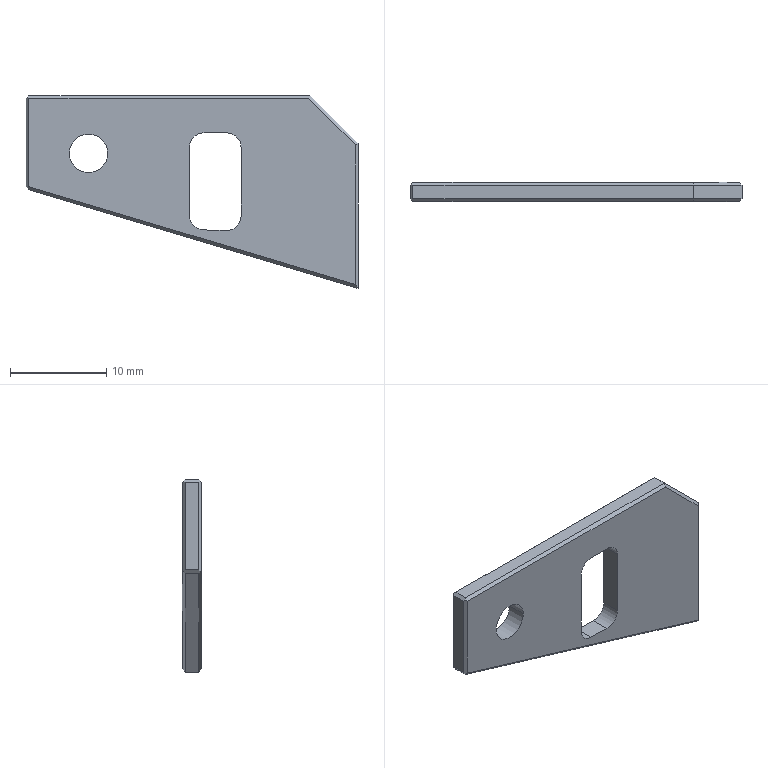Part | NX | 1 solid | 29 faces | box 34.5 x 2 x 20.034 mm | volume 861.777 mm3 | plane 23 | cylinder 6 | commonest cylinder face diameters 3 x4 4 x2
STEP:
#1=CARTESIAN_POINT('',(-158.,158.2,-56.284));
#2=VERTEX_POINT('',#1);
#3=CARTESIAN_POINT('',(-158.,156.8,-56.284));
#4=VERTEX_POINT('',#3);
#5=CARTESIAN_POINT('',(-158.,157.5,-56.284));
#6=DIRECTION('',(0.,-1.,0.));
#7=VECTOR('',#6,1000.);
#8=LINE('',#5,#7);
#9=EDGE_CURVE('',#2,#4,#8,.T.);
#10=ORIENTED_EDGE('',*,*,#9,.T.);
#11=CARTESIAN_POINT('',(-158.,156.8,-47.2));
#12=VERTEX_POINT('',#11);
#13=CARTESIAN_POINT('',(-158.,156.8,-58.685));
#14=DIRECTION('',(0.,0.,1.));
#15=VECTOR('',#14,1000.);
#16=LINE('',#13,#15);
#17=EDGE_CURVE('',#4,#12,#16,.T.);
#18=ORIENTED_EDGE('',*,*,#17,.T.);
#19=CARTESIAN_POINT('',(-158.,158.2,-47.2));
#20=VERTEX_POINT('',#19);
#21=CARTESIAN_POINT('',(-158.,157.5,-47.2));
#22=DIRECTION('',(0.,1.,0.));
#23=VECTOR('',#22,1000.);
#24=LINE('',#21,#23);
#25=EDGE_CURVE('',#12,#20,#24,.T.);
#26=ORIENTED_EDGE('',*,*,#25,.T.);
#27=CARTESIAN_POINT('',(-158.,158.2,-58.685));
#28=DIRECTION('',(0.,0.,1.));
#29=VECTOR('',#28,1000.);
#30=LINE('',#27,#29);
#31=EDGE_CURVE('',#2,#20,#30,.T.);
#32=ORIENTED_EDGE('',*,*,#31,.F.);
#33=EDGE_LOOP('',(#10,#18,#26,#32));
#34=FACE_BOUND('',#33,.T.);
#35=CARTESIAN_POINT('',(-158.,156.5,-42.9));
#36=DIRECTION('',(-1.,0.,0.));
#37=DIRECTION('',(0.,0.,1.));
#38=AXIS2_PLACEMENT_3D('',#35,#36,#37);
#39=PLANE('',#38);
#40=ADVANCED_FACE('',(#34),#39,.T.);
#41=CARTESIAN_POINT('',(-128.5,156.8,-46.9));
#42=VERTEX_POINT('',#41);
#43=CARTESIAN_POINT('',(-128.5,158.2,-46.9));
#44=VERTEX_POINT('',#43);
#45=CARTESIAN_POINT('',(-128.5,157.5,-46.9));
#46=DIRECTION('',(0.,1.,0.));
#47=VECTOR('',#46,1000.);
#48=LINE('',#45,#47);
#49=EDGE_CURVE('',#42,#44,#48,.T.);
#50=ORIENTED_EDGE('',*,*,#49,.T.);
#51=CARTESIAN_POINT('',(-157.7,158.2,-46.9));
#52=VERTEX_POINT('',#51);
#53=CARTESIAN_POINT('',(-143.25,158.2,-46.9));
#54=DIRECTION('',(1.,0.,0.));
#55=VECTOR('',#54,1000.);
#56=LINE('',#53,#55);
#57=EDGE_CURVE('',#52,#44,#56,.T.);
#58=ORIENTED_EDGE('',*,*,#57,.F.);
#59=CARTESIAN_POINT('',(-157.7,156.8,-46.9));
#60=VERTEX_POINT('',#59);
#61=CARTESIAN_POINT('',(-157.7,157.5,-46.9));
#62=DIRECTION('',(0.,1.,0.));
#63=VECTOR('',#62,1000.);
#64=LINE('',#61,#63);
#65=EDGE_CURVE('',#60,#52,#64,.T.);
#66=ORIENTED_EDGE('',*,*,#65,.F.);
#67=CARTESIAN_POINT('',(-143.25,156.8,-46.9));
#68=DIRECTION('',(1.,0.,0.));
#69=VECTOR('',#68,1000.);
#70=LINE('',#67,#69);
#71=EDGE_CURVE('',#60,#42,#70,.T.);
#72=ORIENTED_EDGE('',*,*,#71,.T.);
#73=EDGE_LOOP('',(#50,#58,#66,#72));
#74=FACE_BOUND('',#73,.T.);
#75=CARTESIAN_POINT('',(-123.5,156.5,-46.9));
#76=DIRECTION('',(0.,0.,1.));
#77=DIRECTION('',(0.,-1.,0.));
#78=AXIS2_PLACEMENT_3D('',#75,#76,#77);
#79=PLANE('',#78);
#80=ADVANCED_FACE('',(#74),#79,.T.);
#81=CARTESIAN_POINT('',(-123.5,158.2,-51.9));
#82=VERTEX_POINT('',#81);
#83=CARTESIAN_POINT('',(-123.5,158.2,-66.934));
#84=VERTEX_POINT('',#83);
#85=CARTESIAN_POINT('',(-123.5,158.2,-58.685));
#86=DIRECTION('',(0.,0.,-1.));
#87=VECTOR('',#86,1000.);
#88=LINE('',#85,#87);
#89=EDGE_CURVE('',#82,#84,#88,.T.);
#90=ORIENTED_EDGE('',*,*,#89,.F.);
#91=CARTESIAN_POINT('',(-123.5,156.8,-51.9));
#92=VERTEX_POINT('',#91);
#93=CARTESIAN_POINT('',(-123.5,157.5,-51.9));
#94=DIRECTION('',(0.,1.,0.));
#95=VECTOR('',#94,1000.);
#96=LINE('',#93,#95);
#97=EDGE_CURVE('',#92,#82,#96,.T.);
#98=ORIENTED_EDGE('',*,*,#97,.F.);
#99=CARTESIAN_POINT('',(-123.5,156.8,-66.934));
#100=VERTEX_POINT('',#99);
#101=CARTESIAN_POINT('',(-123.5,156.8,-58.685));
#102=DIRECTION('',(0.,0.,-1.));
#103=VECTOR('',#102,1000.);
#104=LINE('',#101,#103);
#105=EDGE_CURVE('',#92,#100,#104,.T.);
#106=ORIENTED_EDGE('',*,*,#105,.T.);
#107=CARTESIAN_POINT('',(-123.5,156.5,-66.934));
#108=DIRECTION('',(0.,1.,0.));
#109=VECTOR('',#108,1000.);
#110=LINE('',#107,#109);
#111=EDGE_CURVE('',#100,#84,#110,.T.);
#112=ORIENTED_EDGE('',*,*,#111,.T.);
#113=EDGE_LOOP('',(#90,#98,#106,#112));
#114=FACE_BOUND('',#113,.T.);
#115=CARTESIAN_POINT('',(-123.5,156.5,-67.9));
#116=DIRECTION('',(1.,0.,0.));
#117=DIRECTION('',(0.,1.,0.));
#118=AXIS2_PLACEMENT_3D('',#115,#116,#117);
#119=PLANE('',#118);
#120=ADVANCED_FACE('',(#114),#119,.T.);
#121=CARTESIAN_POINT('',(-135.65,156.5,-59.427));
#122=VERTEX_POINT('',#121);
#123=CARTESIAN_POINT('',(-135.65,158.5,-59.427));
#124=VERTEX_POINT('',#123);
#125=CARTESIAN_POINT('',(-135.65,156.5,-59.427));
#126=DIRECTION('',(0.,1.,0.));
#127=VECTOR('',#126,1000.);
#128=LINE('',#125,#127);
#129=EDGE_CURVE('',#122,#124,#128,.T.);
#130=ORIENTED_EDGE('',*,*,#129,.T.);
#131=CARTESIAN_POINT('',(-137.197,158.5,-60.926));
#132=VERTEX_POINT('',#131);
#133=CARTESIAN_POINT('',(-137.15,158.5,-59.427));
#134=DIRECTION('',(0.,1.,0.));
#135=DIRECTION('',(-1.,0.,0.));
#136=AXIS2_PLACEMENT_3D('',#133,#134,#135);
#137=CIRCLE('',#136,1.5);
#138=EDGE_CURVE('',#124,#132,#137,.T.);
#139=ORIENTED_EDGE('',*,*,#138,.T.);
#140=CARTESIAN_POINT('',(-137.197,156.5,-60.926));
#141=VERTEX_POINT('',#140);
#142=CARTESIAN_POINT('',(-137.197,156.5,-60.926));
#143=DIRECTION('',(0.,1.,0.));
#144=VECTOR('',#143,1000.);
#145=LINE('',#142,#144);
#146=EDGE_CURVE('',#141,#132,#145,.T.);
#147=ORIENTED_EDGE('',*,*,#146,.F.);
#148=CARTESIAN_POINT('',(-137.15,156.5,-59.427));
#149=DIRECTION('',(0.,1.,0.));
#150=DIRECTION('',(-1.,0.,0.));
#151=AXIS2_PLACEMENT_3D('',#148,#149,#150);
#152=CIRCLE('',#151,1.5);
#153=EDGE_CURVE('',#122,#141,#152,.T.);
#154=ORIENTED_EDGE('',*,*,#153,.F.);
#155=EDGE_LOOP('',(#130,#139,#147,#154));
#156=FACE_BOUND('',#155,.T.);
#157=CARTESIAN_POINT('',(-137.15,156.5,-59.427));
#158=DIRECTION('',(0.,1.,0.));
#159=DIRECTION('',(-1.,0.,0.));
#160=AXIS2_PLACEMENT_3D('',#157,#158,#159);
#161=CYLINDRICAL_SURFACE('',#160,1.5);
#162=ADVANCED_FACE('',(#156),#161,.F.);
#163=ORIENTED_EDGE('',*,*,#111,.F.);
#164=CARTESIAN_POINT('',(-157.713,156.8,-56.67));
#165=VERTEX_POINT('',#164);
#166=CARTESIAN_POINT('',(-140.75,156.8,-61.759));
#167=DIRECTION('',(-0.9578,0.,0.2873));
#168=VECTOR('',#167,1000.);
#169=LINE('',#166,#168);
#170=EDGE_CURVE('',#100,#165,#169,.T.);
#171=ORIENTED_EDGE('',*,*,#170,.T.);
#172=CARTESIAN_POINT('',(-157.713,158.2,-56.67));
#173=VERTEX_POINT('',#172);
#174=CARTESIAN_POINT('',(-157.713,157.5,-56.67));
#175=DIRECTION('',(0.,-1.,0.));
#176=VECTOR('',#175,1000.);
#177=LINE('',#174,#176);
#178=EDGE_CURVE('',#173,#165,#177,.T.);
#179=ORIENTED_EDGE('',*,*,#178,.F.);
#180=CARTESIAN_POINT('',(-140.75,158.2,-61.759));
#181=DIRECTION('',(-0.9578,0.,0.2873));
#182=VECTOR('',#181,1000.);
#183=LINE('',#180,#182);
#184=EDGE_CURVE('',#84,#173,#183,.T.);
#185=ORIENTED_EDGE('',*,*,#184,.F.);
#186=EDGE_LOOP('',(#163,#171,#179,#185));
#187=FACE_BOUND('',#186,.T.);
#188=CARTESIAN_POINT('',(-160.069,156.5,-55.963));
#189=DIRECTION('',(-0.2873,0.,-0.9578));
#190=DIRECTION('',(-0.9578,0.,0.2873));
#191=AXIS2_PLACEMENT_3D('',#188,#189,#190);
#192=PLANE('',#191);
#193=ADVANCED_FACE('',(#187),#192,.T.);
#194=CARTESIAN_POINT('',(-141.001,156.5,-59.354));
#195=VERTEX_POINT('',#194);
#196=CARTESIAN_POINT('',(-141.001,158.5,-59.354));
#197=VERTEX_POINT('',#196);
#198=CARTESIAN_POINT('',(-141.001,156.5,-59.354));
#199=DIRECTION('',(0.,1.,0.));
#200=VECTOR('',#199,1000.);
#201=LINE('',#198,#200);
#202=EDGE_CURVE('',#195,#197,#201,.T.);
#203=ORIENTED_EDGE('',*,*,#202,.F.);
#204=CARTESIAN_POINT('',(-139.548,156.5,-60.853));
#205=VERTEX_POINT('',#204);
#206=CARTESIAN_POINT('',(-139.501,156.5,-59.354));
#207=DIRECTION('',(0.,1.,0.));
#208=DIRECTION('',(-1.,0.,0.));
#209=AXIS2_PLACEMENT_3D('',#206,#207,#208);
#210=CIRCLE('',#209,1.5);
#211=EDGE_CURVE('',#205,#195,#210,.T.);
#212=ORIENTED_EDGE('',*,*,#211,.F.);
#213=CARTESIAN_POINT('',(-139.548,158.5,-60.853));
#214=VERTEX_POINT('',#213);
#215=CARTESIAN_POINT('',(-139.548,156.5,-60.853));
#216=DIRECTION('',(0.,1.,0.));
#217=VECTOR('',#216,1000.);
#218=LINE('',#215,#217);
#219=EDGE_CURVE('',#205,#214,#218,.T.);
#220=ORIENTED_EDGE('',*,*,#219,.T.);
#221=CARTESIAN_POINT('',(-139.501,158.5,-59.354));
#222=DIRECTION('',(0.,1.,0.));
#223=DIRECTION('',(-1.,0.,0.));
#224=AXIS2_PLACEMENT_3D('',#221,#222,#223);
#225=CIRCLE('',#224,1.5);
#226=EDGE_CURVE('',#214,#197,#225,.T.);
#227=ORIENTED_EDGE('',*,*,#226,.T.);
#228=EDGE_LOOP('',(#203,#212,#220,#227));
#229=FACE_BOUND('',#228,.T.);
#230=CARTESIAN_POINT('',(-139.501,156.5,-59.354));
#231=DIRECTION('',(0.,1.,0.));
#232=DIRECTION('',(-1.,0.,0.));
#233=AXIS2_PLACEMENT_3D('',#230,#231,#232);
#234=CYLINDRICAL_SURFACE('',#233,1.5);
#235=ADVANCED_FACE('',(#229),#234,.F.);
#236=CARTESIAN_POINT('',(-137.15,156.5,-50.763));
#237=VERTEX_POINT('',#236);
#238=CARTESIAN_POINT('',(-137.15,158.5,-50.763));
#239=VERTEX_POINT('',#238);
#240=CARTESIAN_POINT('',(-137.15,156.5,-50.763));
#241=DIRECTION('',(0.,1.,0.));
#242=VECTOR('',#241,1000.);
#243=LINE('',#240,#242);
#244=EDGE_CURVE('',#237,#239,#243,.T.);
#245=ORIENTED_EDGE('',*,*,#244,.F.);
#246=CARTESIAN_POINT('',(-139.501,156.5,-50.763));
#247=VERTEX_POINT('',#246);
#248=CARTESIAN_POINT('',(-108.092,156.5,-50.763));
#249=DIRECTION('',(1.,0.,0.));
#250=VECTOR('',#249,1000.);
#251=LINE('',#248,#250);
#252=EDGE_CURVE('',#247,#237,#251,.T.);
#253=ORIENTED_EDGE('',*,*,#252,.F.);
#254=CARTESIAN_POINT('',(-139.501,158.5,-50.763));
#255=VERTEX_POINT('',#254);
#256=CARTESIAN_POINT('',(-139.501,156.5,-50.763));
#257=DIRECTION('',(0.,1.,0.));
#258=VECTOR('',#257,1000.);
#259=LINE('',#256,#258);
#260=EDGE_CURVE('',#247,#255,#259,.T.);
#261=ORIENTED_EDGE('',*,*,#260,.T.);
#262=CARTESIAN_POINT('',(-108.092,158.5,-50.763));
#263=DIRECTION('',(1.,0.,0.));
#264=VECTOR('',#263,1000.);
#265=LINE('',#262,#264);
#266=EDGE_CURVE('',#255,#239,#265,.T.);
#267=ORIENTED_EDGE('',*,*,#266,.T.);
#268=EDGE_LOOP('',(#245,#253,#261,#267));
#269=FACE_BOUND('',#268,.T.);
#270=CARTESIAN_POINT('',(-135.65,156.3,-50.763));
#271=DIRECTION('',(0.,0.,1.));
#272=DIRECTION('',(0.,-1.,0.));
#273=AXIS2_PLACEMENT_3D('',#270,#271,#272);
#274=PLANE('',#273);
#275=ADVANCED_FACE('',(#269),#274,.F.);
#276=ORIENTED_EDGE('',*,*,#129,.F.);
#277=CARTESIAN_POINT('',(-135.65,156.5,-52.263));
#278=VERTEX_POINT('',#277);
#279=CARTESIAN_POINT('',(-135.65,156.5,-58.685));
#280=DIRECTION('',(0.,0.,-1.));
#281=VECTOR('',#280,1000.);
#282=LINE('',#279,#281);
#283=EDGE_CURVE('',#278,#122,#282,.T.);
#284=ORIENTED_EDGE('',*,*,#283,.F.);
#285=CARTESIAN_POINT('',(-135.65,158.5,-52.263));
#286=VERTEX_POINT('',#285);
#287=CARTESIAN_POINT('',(-135.65,156.5,-52.263));
#288=DIRECTION('',(0.,1.,0.));
#289=VECTOR('',#288,1000.);
#290=LINE('',#287,#289);
#291=EDGE_CURVE('',#278,#286,#290,.T.);
#292=ORIENTED_EDGE('',*,*,#291,.T.);
#293=CARTESIAN_POINT('',(-135.65,158.5,-58.685));
#294=DIRECTION('',(0.,0.,-1.));
#295=VECTOR('',#294,1000.);
#296=LINE('',#293,#295);
#297=EDGE_CURVE('',#286,#124,#296,.T.);
#298=ORIENTED_EDGE('',*,*,#297,.T.);
#299=EDGE_LOOP('',(#276,#284,#292,#298));
#300=FACE_BOUND('',#299,.T.);
#301=CARTESIAN_POINT('',(-135.65,156.3,-60.975));
#302=DIRECTION('',(1.,0.,0.));
#303=DIRECTION('',(0.,0.,-1.));
#304=AXIS2_PLACEMENT_3D('',#301,#302,#303);
#305=PLANE('',#304);
#306=ADVANCED_FACE('',(#300),#305,.F.);
#307=CARTESIAN_POINT('',(-108.092,158.5,-61.836));
#308=DIRECTION('',(-0.9995,0.,0.03124));
#309=VECTOR('',#308,1000.);
#310=LINE('',#307,#309);
#311=EDGE_CURVE('',#132,#214,#310,.T.);
#312=ORIENTED_EDGE('',*,*,#311,.T.);
#313=ORIENTED_EDGE('',*,*,#219,.F.);
#314=CARTESIAN_POINT('',(-108.092,156.5,-61.836));
#315=DIRECTION('',(-0.9995,0.,0.03124));
#316=VECTOR('',#315,1000.);
#317=LINE('',#314,#316);
#318=EDGE_CURVE('',#141,#205,#317,.T.);
#319=ORIENTED_EDGE('',*,*,#318,.F.);
#320=ORIENTED_EDGE('',*,*,#146,.T.);
#321=EDGE_LOOP('',(#312,#313,#319,#320));
#322=FACE_BOUND('',#321,.T.);
#323=CARTESIAN_POINT('',(-141.001,156.3,-60.807));
#324=DIRECTION('',(-0.03124,0.,-0.9995));
#325=DIRECTION('',(-0.9995,0.,0.03124));
#326=AXIS2_PLACEMENT_3D('',#323,#324,#325);
#327=PLANE('',#326);
#328=ADVANCED_FACE('',(#322),#327,.F.);
#329=ORIENTED_EDGE('',*,*,#202,.T.);
#330=CARTESIAN_POINT('',(-141.001,158.5,-52.263));
#331=VERTEX_POINT('',#330);
#332=CARTESIAN_POINT('',(-141.001,158.5,-58.685));
#333=DIRECTION('',(0.,0.,1.));
#334=VECTOR('',#333,1000.);
#335=LINE('',#332,#334);
#336=EDGE_CURVE('',#197,#331,#335,.T.);
#337=ORIENTED_EDGE('',*,*,#336,.T.);
#338=CARTESIAN_POINT('',(-141.001,156.5,-52.263));
#339=VERTEX_POINT('',#338);
#340=CARTESIAN_POINT('',(-141.001,156.5,-52.263));
#341=DIRECTION('',(0.,1.,0.));
#342=VECTOR('',#341,1000.);
#343=LINE('',#340,#342);
#344=EDGE_CURVE('',#339,#331,#343,.T.);
#345=ORIENTED_EDGE('',*,*,#344,.F.);
#346=CARTESIAN_POINT('',(-141.001,156.5,-58.685));
#347=DIRECTION('',(0.,0.,1.));
#348=VECTOR('',#347,1000.);
#349=LINE('',#346,#348);
#350=EDGE_CURVE('',#195,#339,#349,.T.);
#351=ORIENTED_EDGE('',*,*,#350,.F.);
#352=EDGE_LOOP('',(#329,#337,#345,#351));
#353=FACE_BOUND('',#352,.T.);
#354=CARTESIAN_POINT('',(-141.001,156.3,-50.763));
#355=DIRECTION('',(-1.,0.,0.));
#356=DIRECTION('',(0.,0.,1.));
#357=AXIS2_PLACEMENT_3D('',#354,#355,#356);
#358=PLANE('',#357);
#359=ADVANCED_FACE('',(#353),#358,.F.);
#360=ORIENTED_EDGE('',*,*,#344,.T.);
#361=CARTESIAN_POINT('',(-139.501,158.5,-52.263));
#362=DIRECTION('',(0.,1.,0.));
#363=DIRECTION('',(-1.,0.,0.));
#364=AXIS2_PLACEMENT_3D('',#361,#362,#363);
#365=CIRCLE('',#364,1.5);
#366=EDGE_CURVE('',#331,#255,#365,.T.);
#367=ORIENTED_EDGE('',*,*,#366,.T.);
#368=ORIENTED_EDGE('',*,*,#260,.F.);
#369=CARTESIAN_POINT('',(-139.501,156.5,-52.263));
#370=DIRECTION('',(0.,1.,0.));
#371=DIRECTION('',(-1.,0.,0.));
#372=AXIS2_PLACEMENT_3D('',#369,#370,#371);
#373=CIRCLE('',#372,1.5);
#374=EDGE_CURVE('',#339,#247,#373,.T.);
#375=ORIENTED_EDGE('',*,*,#374,.F.);
#376=EDGE_LOOP('',(#360,#367,#368,#375));
#377=FACE_BOUND('',#376,.T.);
#378=CARTESIAN_POINT('',(-139.501,156.5,-52.263));
#379=DIRECTION('',(0.,1.,0.));
#380=DIRECTION('',(-1.,0.,0.));
#381=AXIS2_PLACEMENT_3D('',#378,#379,#380);
#382=CYLINDRICAL_SURFACE('',#381,1.5);
#383=ADVANCED_FACE('',(#377),#382,.F.);
#384=ORIENTED_EDGE('',*,*,#244,.T.);
#385=CARTESIAN_POINT('',(-137.15,158.5,-52.263));
#386=DIRECTION('',(0.,1.,0.));
#387=DIRECTION('',(-1.,0.,0.));
#388=AXIS2_PLACEMENT_3D('',#385,#386,#387);
#389=CIRCLE('',#388,1.5);
#390=EDGE_CURVE('',#239,#286,#389,.T.);
#391=ORIENTED_EDGE('',*,*,#390,.T.);
#392=ORIENTED_EDGE('',*,*,#291,.F.);
#393=CARTESIAN_POINT('',(-137.15,156.5,-52.263));
#394=DIRECTION('',(0.,1.,0.));
#395=DIRECTION('',(-1.,0.,0.));
#396=AXIS2_PLACEMENT_3D('',#393,#394,#395);
#397=CIRCLE('',#396,1.5);
#398=EDGE_CURVE('',#237,#278,#397,.T.);
#399=ORIENTED_EDGE('',*,*,#398,.F.);
#400=EDGE_LOOP('',(#384,#391,#392,#399));
#401=FACE_BOUND('',#400,.T.);
#402=CARTESIAN_POINT('',(-137.15,156.5,-52.263));
#403=DIRECTION('',(0.,1.,0.));
#404=DIRECTION('',(-1.,0.,0.));
#405=AXIS2_PLACEMENT_3D('',#402,#403,#404);
#406=CYLINDRICAL_SURFACE('',#405,1.5);
#407=ADVANCED_FACE('',(#401),#406,.F.);
#408=CARTESIAN_POINT('',(-126.,158.2,-49.4));
#409=DIRECTION('',(-0.7071,0.,0.7071));
#410=VECTOR('',#409,1000.);
#411=LINE('',#408,#410);
#412=EDGE_CURVE('',#82,#44,#411,.T.);
#413=ORIENTED_EDGE('',*,*,#412,.T.);
#414=ORIENTED_EDGE('',*,*,#49,.F.);
#415=CARTESIAN_POINT('',(-126.,156.8,-49.4));
#416=DIRECTION('',(-0.7071,0.,0.7071));
#417=VECTOR('',#416,1000.);
#418=LINE('',#415,#417);
#419=EDGE_CURVE('',#92,#42,#418,.T.);
#420=ORIENTED_EDGE('',*,*,#419,.F.);
#421=ORIENTED_EDGE('',*,*,#97,.T.);
#422=EDGE_LOOP('',(#413,#414,#420,#421));
#423=FACE_BOUND('',#422,.T.);
#424=CARTESIAN_POINT('',(-126.,157.5,-49.4));
#425=DIRECTION('',(0.7071,0.,0.7071));
#426=DIRECTION('',(0.,-1.,0.));
#427=AXIS2_PLACEMENT_3D('',#424,#425,#426);
#428=PLANE('',#427);
#429=ADVANCED_FACE('',(#423),#428,.T.);
#430=ORIENTED_EDGE('',*,*,#412,.F.);
#431=CARTESIAN_POINT('',(-123.8,158.5,-52.024));
#432=VERTEX_POINT('',#431);
#433=CARTESIAN_POINT('',(-108.092,142.792,-45.518));
#434=DIRECTION('',(0.6786,-0.6786,0.2811));
#435=VECTOR('',#434,1000.);
#436=LINE('',#433,#435);
#437=EDGE_CURVE('',#432,#82,#436,.T.);
#438=ORIENTED_EDGE('',*,*,#437,.F.);
#439=CARTESIAN_POINT('',(-128.624,158.5,-47.2));
#440=VERTEX_POINT('',#439);
#441=CARTESIAN_POINT('',(-126.212,158.5,-49.612));
#442=DIRECTION('',(-0.7071,0.,0.7071));
#443=VECTOR('',#442,1000.);
#444=LINE('',#441,#443);
#445=EDGE_CURVE('',#432,#440,#444,.T.);
#446=ORIENTED_EDGE('',*,*,#445,.T.);
#447=CARTESIAN_POINT('',(-133.381,169.985,-58.685));
#448=DIRECTION('',(-0.2811,0.6786,-0.6786));
#449=VECTOR('',#448,1000.);
#450=LINE('',#447,#449);
#451=EDGE_CURVE('',#44,#440,#450,.T.);
#452=ORIENTED_EDGE('',*,*,#451,.F.);
#453=EDGE_LOOP('',(#430,#438,#446,#452));
#454=FACE_BOUND('',#453,.T.);
#455=CARTESIAN_POINT('',(-126.106,158.35,-49.506));
#456=DIRECTION('',(0.5,0.7071,0.5));
#457=DIRECTION('',(0.7071,0.,-0.7071));
#458=AXIS2_PLACEMENT_3D('',#455,#456,#457);
#459=PLANE('',#458);
#460=ADVANCED_FACE('',(#454),#459,.T.);
#461=ORIENTED_EDGE('',*,*,#25,.F.);
#462=CARTESIAN_POINT('',(-157.85,156.65,-47.05));
#463=VERTEX_POINT('',#462);
#464=CARTESIAN_POINT('',(-169.485,168.285,-58.685));
#465=DIRECTION('',(0.5774,-0.5774,0.5774));
#466=VECTOR('',#465,1000.);
#467=LINE('',#464,#466);
#468=EDGE_CURVE('',#12,#463,#467,.T.);
#469=ORIENTED_EDGE('',*,*,#468,.T.);
#470=CARTESIAN_POINT('',(-169.485,145.015,-58.685));
#471=DIRECTION('',(0.5774,0.5774,0.5774));
#472=VECTOR('',#471,1000.);
#473=LINE('',#470,#472);
#474=EDGE_CURVE('',#463,#60,#473,.T.);
#475=ORIENTED_EDGE('',*,*,#474,.T.);
#476=ORIENTED_EDGE('',*,*,#65,.T.);
#477=CARTESIAN_POINT('',(-157.85,158.35,-47.05));
#478=VERTEX_POINT('',#477);
#479=CARTESIAN_POINT('',(-169.485,169.985,-58.685));
#480=DIRECTION('',(0.5774,-0.5774,0.5774));
#481=VECTOR('',#480,1000.);
#482=LINE('',#479,#481);
#483=EDGE_CURVE('',#478,#52,#482,.T.);
#484=ORIENTED_EDGE('',*,*,#483,.F.);
#485=CARTESIAN_POINT('',(-169.485,146.715,-58.685));
#486=DIRECTION('',(0.5774,0.5774,0.5774));
#487=VECTOR('',#486,1000.);
#488=LINE('',#485,#487);
#489=EDGE_CURVE('',#20,#478,#488,.T.);
#490=ORIENTED_EDGE('',*,*,#489,.F.);
#491=EDGE_LOOP('',(#461,#469,#475,#476,#484,#490));
#492=FACE_BOUND('',#491,.T.);
#493=CARTESIAN_POINT('',(-157.85,157.5,-47.05));
#494=DIRECTION('',(-0.7071,0.,0.7071));
#495=DIRECTION('',(0.,1.,0.));
#496=AXIS2_PLACEMENT_3D('',#493,#494,#495);
#497=PLANE('',#496);
#498=ADVANCED_FACE('',(#492),#497,.T.);
#499=ORIENTED_EDGE('',*,*,#419,.T.);
#500=CARTESIAN_POINT('',(-128.624,156.5,-47.2));
#501=VERTEX_POINT('',#500);
#502=CARTESIAN_POINT('',(-133.381,145.015,-58.685));
#503=DIRECTION('',(0.2811,0.6786,0.6786));
#504=VECTOR('',#503,1000.);
#505=LINE('',#502,#504);
#506=EDGE_CURVE('',#501,#42,#505,.T.);
#507=ORIENTED_EDGE('',*,*,#506,.F.);
#508=CARTESIAN_POINT('',(-123.8,156.5,-52.024));
#509=VERTEX_POINT('',#508);
#510=CARTESIAN_POINT('',(-126.212,156.5,-49.612));
#511=DIRECTION('',(-0.7071,0.,0.7071));
#512=VECTOR('',#511,1000.);
#513=LINE('',#510,#512);
#514=EDGE_CURVE('',#509,#501,#513,.T.);
#515=ORIENTED_EDGE('',*,*,#514,.F.);
#516=CARTESIAN_POINT('',(-108.092,172.208,-45.518));
#517=DIRECTION('',(-0.6786,-0.6786,-0.2811));
#518=VECTOR('',#517,1000.);
#519=LINE('',#516,#518);
#520=EDGE_CURVE('',#92,#509,#519,.T.);
#521=ORIENTED_EDGE('',*,*,#520,.F.);
#522=EDGE_LOOP('',(#499,#507,#515,#521));
#523=FACE_BOUND('',#522,.T.);
#524=CARTESIAN_POINT('',(-126.106,156.65,-49.506));
#525=DIRECTION('',(-0.5,0.7071,-0.5));
#526=DIRECTION('',(-0.7071,0.,0.7071));
#527=AXIS2_PLACEMENT_3D('',#524,#525,#526);
#528=PLANE('',#527);
#529=ADVANCED_FACE('',(#523),#528,.F.);
#530=ORIENTED_EDGE('',*,*,#9,.F.);
#531=CARTESIAN_POINT('',(-157.856,158.344,-56.477));
#532=VERTEX_POINT('',#531);
#533=CARTESIAN_POINT('',(-156.214,159.986,-58.685));
#534=DIRECTION('',(0.5126,0.5126,-0.6889));
#535=VECTOR('',#534,1000.);
#536=LINE('',#533,#535);
#537=EDGE_CURVE('',#2,#532,#536,.T.);
#538=ORIENTED_EDGE('',*,*,#537,.T.);
#539=CARTESIAN_POINT('',(-156.214,156.701,-58.685));
#540=DIRECTION('',(-0.5126,0.5126,0.6889));
#541=VECTOR('',#540,1000.);
#542=LINE('',#539,#541);
#543=EDGE_CURVE('',#173,#532,#542,.T.);
#544=ORIENTED_EDGE('',*,*,#543,.F.);
#545=ORIENTED_EDGE('',*,*,#178,.T.);
#546=CARTESIAN_POINT('',(-157.856,156.656,-56.477));
#547=VERTEX_POINT('',#546);
#548=CARTESIAN_POINT('',(-156.214,158.299,-58.685));
#549=DIRECTION('',(0.5126,0.5126,-0.6889));
#550=VECTOR('',#549,1000.);
#551=LINE('',#548,#550);
#552=EDGE_CURVE('',#547,#165,#551,.T.);
#553=ORIENTED_EDGE('',*,*,#552,.F.);
#554=CARTESIAN_POINT('',(-156.214,155.014,-58.685));
#555=DIRECTION('',(0.5126,-0.5126,-0.6889));
#556=VECTOR('',#555,1000.);
#557=LINE('',#554,#556);
#558=EDGE_CURVE('',#4,#547,#557,.T.);
#559=ORIENTED_EDGE('',*,*,#558,.F.);
#560=EDGE_LOOP('',(#530,#538,#544,#545,#553,#559));
#561=FACE_BOUND('',#560,.T.);
#562=CARTESIAN_POINT('',(-157.856,157.5,-56.477));
#563=DIRECTION('',(-0.8023,0.,-0.5969));
#564=DIRECTION('',(-0.5969,0.,0.8023));
#565=AXIS2_PLACEMENT_3D('',#562,#563,#564);
#566=PLANE('',#565);
#567=ADVANCED_FACE('',(#561),#566,.T.);
#568=CARTESIAN_POINT('',(-149.5,158.5,-52.9));
#569=VERTEX_POINT('',#568);
#570=CARTESIAN_POINT('',(-153.5,158.5,-52.9));
#571=VERTEX_POINT('',#570);
#572=CARTESIAN_POINT('',(-151.5,158.5,-52.9));
#573=DIRECTION('',(0.,1.,0.));
#574=DIRECTION('',(-1.,0.,0.));
#575=AXIS2_PLACEMENT_3D('',#572,#573,#574);
#576=CIRCLE('',#575,2.);
#577=EDGE_CURVE('',#569,#571,#576,.T.);
#578=ORIENTED_EDGE('',*,*,#577,.T.);
#579=CARTESIAN_POINT('',(-153.5,156.5,-52.9));
#580=VERTEX_POINT('',#579);
#581=CARTESIAN_POINT('',(-153.5,156.5,-52.9));
#582=DIRECTION('',(0.,1.,0.));
#583=VECTOR('',#582,1000.);
#584=LINE('',#581,#583);
#585=EDGE_CURVE('',#571,#580,#584,.F.);
#586=ORIENTED_EDGE('',*,*,#585,.T.);
#587=CARTESIAN_POINT('',(-149.5,156.5,-52.9));
#588=VERTEX_POINT('',#587);
#589=CARTESIAN_POINT('',(-151.5,156.5,-52.9));
#590=DIRECTION('',(0.,1.,0.));
#591=DIRECTION('',(-1.,0.,0.));
#592=AXIS2_PLACEMENT_3D('',#589,#590,#591);
#593=CIRCLE('',#592,2.);
#594=EDGE_CURVE('',#588,#580,#593,.T.);
#595=ORIENTED_EDGE('',*,*,#594,.F.);
#596=CARTESIAN_POINT('',(-149.5,156.5,-52.9));
#597=DIRECTION('',(0.,1.,0.));
#598=VECTOR('',#597,1000.);
#599=LINE('',#596,#598);
#600=EDGE_CURVE('',#569,#588,#599,.F.);
#601=ORIENTED_EDGE('',*,*,#600,.F.);
#602=EDGE_LOOP('',(#578,#586,#595,#601));
#603=FACE_BOUND('',#602,.T.);
#604=CARTESIAN_POINT('',(-151.5,156.5,-52.9));
#605=DIRECTION('',(0.,1.,0.));
#606=DIRECTION('',(-1.,0.,0.));
#607=AXIS2_PLACEMENT_3D('',#604,#605,#606);
#608=CYLINDRICAL_SURFACE('',#607,2.);
#609=ADVANCED_FACE('',(#603),#608,.F.);
#610=ORIENTED_EDGE('',*,*,#585,.F.);
#611=CARTESIAN_POINT('',(-151.5,158.5,-52.9));
#612=DIRECTION('',(0.,1.,0.));
#613=DIRECTION('',(-1.,0.,0.));
#614=AXIS2_PLACEMENT_3D('',#611,#612,#613);
#615=CIRCLE('',#614,2.);
#616=EDGE_CURVE('',#571,#569,#615,.T.);
#617=ORIENTED_EDGE('',*,*,#616,.T.);
#618=ORIENTED_EDGE('',*,*,#600,.T.);
#619=CARTESIAN_POINT('',(-151.5,156.5,-52.9));
#620=DIRECTION('',(0.,1.,0.));
#621=DIRECTION('',(-1.,0.,0.));
#622=AXIS2_PLACEMENT_3D('',#619,#620,#621);
#623=CIRCLE('',#622,2.);
#624=EDGE_CURVE('',#580,#588,#623,.T.);
#625=ORIENTED_EDGE('',*,*,#624,.F.);
#626=EDGE_LOOP('',(#610,#617,#618,#625));
#627=FACE_BOUND('',#626,.T.);
#628=CARTESIAN_POINT('',(-151.5,156.5,-52.9));
#629=DIRECTION('',(0.,1.,0.));
#630=DIRECTION('',(-1.,0.,0.));
#631=AXIS2_PLACEMENT_3D('',#628,#629,#630);
#632=CYLINDRICAL_SURFACE('',#631,2.);
#633=ADVANCED_FACE('',(#627),#632,.F.);
#634=CARTESIAN_POINT('',(-123.8,158.5,-66.531));
#635=VERTEX_POINT('',#634);
#636=CARTESIAN_POINT('',(-157.7,158.5,-56.361));
#637=VERTEX_POINT('',#636);
#638=CARTESIAN_POINT('',(-140.664,158.5,-61.472));
#639=DIRECTION('',(-0.9578,0.,0.2873));
#640=VECTOR('',#639,1000.);
#641=LINE('',#638,#640);
#642=EDGE_CURVE('',#635,#637,#641,.T.);
#643=ORIENTED_EDGE('',*,*,#642,.T.);
#644=CARTESIAN_POINT('',(-157.7,158.5,-47.2));
#645=VERTEX_POINT('',#644);
#646=CARTESIAN_POINT('',(-157.7,158.5,-58.685));
#647=DIRECTION('',(0.,0.,1.));
#648=VECTOR('',#647,1000.);
#649=LINE('',#646,#648);
#650=EDGE_CURVE('',#637,#645,#649,.T.);
#651=ORIENTED_EDGE('',*,*,#650,.T.);
#652=CARTESIAN_POINT('',(-143.25,158.5,-47.2));
#653=DIRECTION('',(1.,0.,0.));
#654=VECTOR('',#653,1000.);
#655=LINE('',#652,#654);
#656=EDGE_CURVE('',#645,#440,#655,.T.);
#657=ORIENTED_EDGE('',*,*,#656,.T.);
#658=ORIENTED_EDGE('',*,*,#445,.F.);
#659=CARTESIAN_POINT('',(-123.8,158.5,-58.685));
#660=DIRECTION('',(0.,0.,-1.));
#661=VECTOR('',#660,1000.);
#662=LINE('',#659,#661);
#663=EDGE_CURVE('',#432,#635,#662,.T.);
#664=ORIENTED_EDGE('',*,*,#663,.T.);
#665=EDGE_LOOP('',(#643,#651,#657,#658,#664));
#666=FACE_BOUND('',#665,.T.);
#667=ORIENTED_EDGE('',*,*,#336,.F.);
#668=ORIENTED_EDGE('',*,*,#226,.F.);
#669=ORIENTED_EDGE('',*,*,#311,.F.);
#670=ORIENTED_EDGE('',*,*,#138,.F.);
#671=ORIENTED_EDGE('',*,*,#297,.F.);
#672=ORIENTED_EDGE('',*,*,#390,.F.);
#673=ORIENTED_EDGE('',*,*,#266,.F.);
#674=ORIENTED_EDGE('',*,*,#366,.F.);
#675=EDGE_LOOP('',(#667,#668,#669,#670,#671,#672,#673,#674));
#676=FACE_BOUND('',#675,.T.);
#677=ORIENTED_EDGE('',*,*,#577,.F.);
#678=ORIENTED_EDGE('',*,*,#616,.F.);
#679=EDGE_LOOP('',(#677,#678));
#680=FACE_BOUND('',#679,.T.);
#681=CARTESIAN_POINT('',(-108.092,158.5,-58.685));
#682=DIRECTION('',(0.,1.,0.));
#683=DIRECTION('',(0.,0.,-1.));
#684=AXIS2_PLACEMENT_3D('',#681,#682,#683);
#685=PLANE('',#684);
#686=ADVANCED_FACE('',(#666,#676,#680),#685,.T.);
#687=ORIENTED_EDGE('',*,*,#89,.T.);
#688=CARTESIAN_POINT('',(-129.638,164.338,-58.685));
#689=DIRECTION('',(0.5126,-0.5126,-0.6889));
#690=VECTOR('',#689,1000.);
#691=LINE('',#688,#690);
#692=EDGE_CURVE('',#635,#84,#691,.T.);
#693=ORIENTED_EDGE('',*,*,#692,.F.);
#694=ORIENTED_EDGE('',*,*,#663,.F.);
#695=ORIENTED_EDGE('',*,*,#437,.T.);
#696=EDGE_LOOP('',(#687,#693,#694,#695));
#697=FACE_BOUND('',#696,.T.);
#698=CARTESIAN_POINT('',(-123.65,158.35,-60.2));
#699=DIRECTION('',(0.7071,0.7071,0.));
#700=DIRECTION('',(0.,0.,-1.));
#701=AXIS2_PLACEMENT_3D('',#698,#699,#700);
#702=PLANE('',#701);
#703=ADVANCED_FACE('',(#697),#702,.T.);
#704=ORIENTED_EDGE('',*,*,#656,.F.);
#705=CARTESIAN_POINT('',(-146.215,169.985,-58.685));
#706=DIRECTION('',(-0.5774,-0.5774,0.5774));
#707=VECTOR('',#706,1000.);
#708=LINE('',#705,#707);
#709=EDGE_CURVE('',#645,#478,#708,.T.);
#710=ORIENTED_EDGE('',*,*,#709,.T.);
#711=ORIENTED_EDGE('',*,*,#483,.T.);
#712=ORIENTED_EDGE('',*,*,#57,.T.);
#713=ORIENTED_EDGE('',*,*,#451,.T.);
#714=EDGE_LOOP('',(#704,#710,#711,#712,#713));
#715=FACE_BOUND('',#714,.T.);
#716=CARTESIAN_POINT('',(-143.25,158.35,-47.05));
#717=DIRECTION('',(0.,0.7071,0.7071));
#718=DIRECTION('',(1.,0.,0.));
#719=AXIS2_PLACEMENT_3D('',#716,#717,#718);
#720=PLANE('',#719);
#721=ADVANCED_FACE('',(#715),#720,.T.);
#722=ORIENTED_EDGE('',*,*,#650,.F.);
#723=CARTESIAN_POINT('',(-159.7,156.5,-57.849));
#724=DIRECTION('',(0.6258,0.6258,0.4656));
#725=VECTOR('',#724,1000.);
#726=LINE('',#723,#725);
#727=EDGE_CURVE('',#532,#637,#726,.T.);
#728=ORIENTED_EDGE('',*,*,#727,.F.);
#729=ORIENTED_EDGE('',*,*,#537,.F.);
#730=ORIENTED_EDGE('',*,*,#31,.T.);
#731=ORIENTED_EDGE('',*,*,#489,.T.);
#732=ORIENTED_EDGE('',*,*,#709,.F.);
#733=EDGE_LOOP('',(#722,#728,#729,#730,#731,#732));
#734=FACE_BOUND('',#733,.T.);
#735=CARTESIAN_POINT('',(-157.85,158.35,-52.525));
#736=DIRECTION('',(-0.7071,0.7071,0.));
#737=DIRECTION('',(0.,0.,1.));
#738=AXIS2_PLACEMENT_3D('',#735,#736,#737);
#739=PLANE('',#738);
#740=ADVANCED_FACE('',(#734),#739,.T.);
#741=ORIENTED_EDGE('',*,*,#642,.F.);
#742=ORIENTED_EDGE('',*,*,#692,.T.);
#743=ORIENTED_EDGE('',*,*,#184,.T.);
#744=ORIENTED_EDGE('',*,*,#543,.T.);
#745=ORIENTED_EDGE('',*,*,#727,.T.);
#746=EDGE_LOOP('',(#741,#742,#743,#744,#745));
#747=FACE_BOUND('',#746,.T.);
#748=CARTESIAN_POINT('',(-140.707,158.35,-61.615));
#749=DIRECTION('',(-0.2032,0.7071,-0.6773));
#750=DIRECTION('',(-0.9578,0.,0.2873));
#751=AXIS2_PLACEMENT_3D('',#748,#749,#750);
#752=PLANE('',#751);
#753=ADVANCED_FACE('',(#747),#752,.T.);
#754=CARTESIAN_POINT('',(-123.8,156.5,-66.531));
#755=VERTEX_POINT('',#754);
#756=CARTESIAN_POINT('',(-157.7,156.5,-56.361));
#757=VERTEX_POINT('',#756);
#758=CARTESIAN_POINT('',(-140.664,156.5,-61.472));
#759=DIRECTION('',(-0.9578,0.,0.2873));
#760=VECTOR('',#759,1000.);
#761=LINE('',#758,#760);
#762=EDGE_CURVE('',#755,#757,#761,.T.);
#763=ORIENTED_EDGE('',*,*,#762,.F.);
#764=CARTESIAN_POINT('',(-123.8,156.5,-58.685));
#765=DIRECTION('',(0.,0.,-1.));
#766=VECTOR('',#765,1000.);
#767=LINE('',#764,#766);
#768=EDGE_CURVE('',#509,#755,#767,.T.);
#769=ORIENTED_EDGE('',*,*,#768,.F.);
#770=ORIENTED_EDGE('',*,*,#514,.T.);
#771=CARTESIAN_POINT('',(-157.7,156.5,-47.2));
#772=VERTEX_POINT('',#771);
#773=CARTESIAN_POINT('',(-143.25,156.5,-47.2));
#774=DIRECTION('',(1.,0.,0.));
#775=VECTOR('',#774,1000.);
#776=LINE('',#773,#775);
#777=EDGE_CURVE('',#772,#501,#776,.T.);
#778=ORIENTED_EDGE('',*,*,#777,.F.);
#779=CARTESIAN_POINT('',(-157.7,156.5,-58.685));
#780=DIRECTION('',(0.,0.,1.));
#781=VECTOR('',#780,1000.);
#782=LINE('',#779,#781);
#783=EDGE_CURVE('',#757,#772,#782,.T.);
#784=ORIENTED_EDGE('',*,*,#783,.F.);
#785=EDGE_LOOP('',(#763,#769,#770,#778,#784));
#786=FACE_BOUND('',#785,.T.);
#787=ORIENTED_EDGE('',*,*,#350,.T.);
#788=ORIENTED_EDGE('',*,*,#374,.T.);
#789=ORIENTED_EDGE('',*,*,#252,.T.);
#790=ORIENTED_EDGE('',*,*,#398,.T.);
#791=ORIENTED_EDGE('',*,*,#283,.T.);
#792=ORIENTED_EDGE('',*,*,#153,.T.);
#793=ORIENTED_EDGE('',*,*,#318,.T.);
#794=ORIENTED_EDGE('',*,*,#211,.T.);
#795=EDGE_LOOP('',(#787,#788,#789,#790,#791,#792,#793,#794));
#796=FACE_BOUND('',#795,.T.);
#797=ORIENTED_EDGE('',*,*,#594,.T.);
#798=ORIENTED_EDGE('',*,*,#624,.T.);
#799=EDGE_LOOP('',(#797,#798));
#800=FACE_BOUND('',#799,.T.);
#801=CARTESIAN_POINT('',(-108.092,156.5,-58.685));
#802=DIRECTION('',(0.,1.,0.));
#803=DIRECTION('',(0.,0.,-1.));
#804=AXIS2_PLACEMENT_3D('',#801,#802,#803);
#805=PLANE('',#804);
#806=ADVANCED_FACE('',(#786,#796,#800),#805,.F.);
#807=CARTESIAN_POINT('',(-129.638,150.662,-58.685));
#808=DIRECTION('',(-0.5126,-0.5126,0.6889));
#809=VECTOR('',#808,1000.);
#810=LINE('',#807,#809);
#811=EDGE_CURVE('',#100,#755,#810,.T.);
#812=ORIENTED_EDGE('',*,*,#811,.F.);
#813=ORIENTED_EDGE('',*,*,#105,.F.);
#814=ORIENTED_EDGE('',*,*,#520,.T.);
#815=ORIENTED_EDGE('',*,*,#768,.T.);
#816=EDGE_LOOP('',(#812,#813,#814,#815));
#817=FACE_BOUND('',#816,.T.);
#818=CARTESIAN_POINT('',(-123.65,156.65,-60.2));
#819=DIRECTION('',(-0.7071,0.7071,0.));
#820=DIRECTION('',(0.,0.,1.));
#821=AXIS2_PLACEMENT_3D('',#818,#819,#820);
#822=PLANE('',#821);
#823=ADVANCED_FACE('',(#817),#822,.F.);
#824=ORIENTED_EDGE('',*,*,#777,.T.);
#825=ORIENTED_EDGE('',*,*,#506,.T.);
#826=ORIENTED_EDGE('',*,*,#71,.F.);
#827=ORIENTED_EDGE('',*,*,#474,.F.);
#828=CARTESIAN_POINT('',(-146.215,145.015,-58.685));
#829=DIRECTION('',(0.5774,-0.5774,-0.5774));
#830=VECTOR('',#829,1000.);
#831=LINE('',#828,#830);
#832=EDGE_CURVE('',#463,#772,#831,.T.);
#833=ORIENTED_EDGE('',*,*,#832,.T.);
#834=EDGE_LOOP('',(#824,#825,#826,#827,#833));
#835=FACE_BOUND('',#834,.T.);
#836=CARTESIAN_POINT('',(-143.25,156.65,-47.05));
#837=DIRECTION('',(0.,0.7071,-0.7071));
#838=DIRECTION('',(-1.,0.,0.));
#839=AXIS2_PLACEMENT_3D('',#836,#837,#838);
#840=PLANE('',#839);
#841=ADVANCED_FACE('',(#835),#840,.F.);
#842=ORIENTED_EDGE('',*,*,#17,.F.);
#843=ORIENTED_EDGE('',*,*,#558,.T.);
#844=CARTESIAN_POINT('',(-157.7,156.5,-56.361));
#845=DIRECTION('',(-0.6258,0.6258,-0.4656));
#846=VECTOR('',#845,1000.);
#847=LINE('',#844,#846);
#848=EDGE_CURVE('',#757,#547,#847,.T.);
#849=ORIENTED_EDGE('',*,*,#848,.F.);
#850=ORIENTED_EDGE('',*,*,#783,.T.);
#851=ORIENTED_EDGE('',*,*,#832,.F.);
#852=ORIENTED_EDGE('',*,*,#468,.F.);
#853=EDGE_LOOP('',(#842,#843,#849,#850,#851,#852));
#854=FACE_BOUND('',#853,.T.);
#855=CARTESIAN_POINT('',(-157.85,156.65,-52.525));
#856=DIRECTION('',(0.7071,0.7071,0.));
#857=DIRECTION('',(0.,0.,-1.));
#858=AXIS2_PLACEMENT_3D('',#855,#856,#857);
#859=PLANE('',#858);
#860=ADVANCED_FACE('',(#854),#859,.F.);
#861=ORIENTED_EDGE('',*,*,#762,.T.);
#862=ORIENTED_EDGE('',*,*,#848,.T.);
#863=ORIENTED_EDGE('',*,*,#552,.T.);
#864=ORIENTED_EDGE('',*,*,#170,.F.);
#865=ORIENTED_EDGE('',*,*,#811,.T.);
#866=EDGE_LOOP('',(#861,#862,#863,#864,#865));
#867=FACE_BOUND('',#866,.T.);
#868=CARTESIAN_POINT('',(-140.707,156.65,-61.615));
#869=DIRECTION('',(0.2032,0.7071,0.6773));
#870=DIRECTION('',(0.9578,0.,-0.2873));
#871=AXIS2_PLACEMENT_3D('',#868,#869,#870);
#872=PLANE('',#871);
#873=ADVANCED_FACE('',(#867),#872,.F.);
#874=CLOSED_SHELL('',(#40,#80,#120,#162,#193,#235,#275,#306,#328,#359,#383,#407,#429,#460,#498,#529,#567,#609,#633,#686,#703,#721,#740,#753,#806,#823,#841,#860,#873));
#875=MANIFOLD_SOLID_BREP('',#874);
#876=(LENGTH_UNIT()NAMED_UNIT(*)SI_UNIT(.MILLI.,.METRE.));
#877=UNCERTAINTY_MEASURE_WITH_UNIT(LENGTH_MEASURE(0.00001),#876,'','');
#878=(NAMED_UNIT(*)PLANE_ANGLE_UNIT()SI_UNIT($,.RADIAN.));
#879=(NAMED_UNIT(*)SI_UNIT($,.STERADIAN.)SOLID_ANGLE_UNIT());
#880=(GEOMETRIC_REPRESENTATION_CONTEXT(3)GLOBAL_UNCERTAINTY_ASSIGNED_CONTEXT((#877))GLOBAL_UNIT_ASSIGNED_CONTEXT((#876,#878,#879))REPRESENTATION_CONTEXT('',''));
#881=ADVANCED_BREP_SHAPE_REPRESENTATION('',(#875),#880);